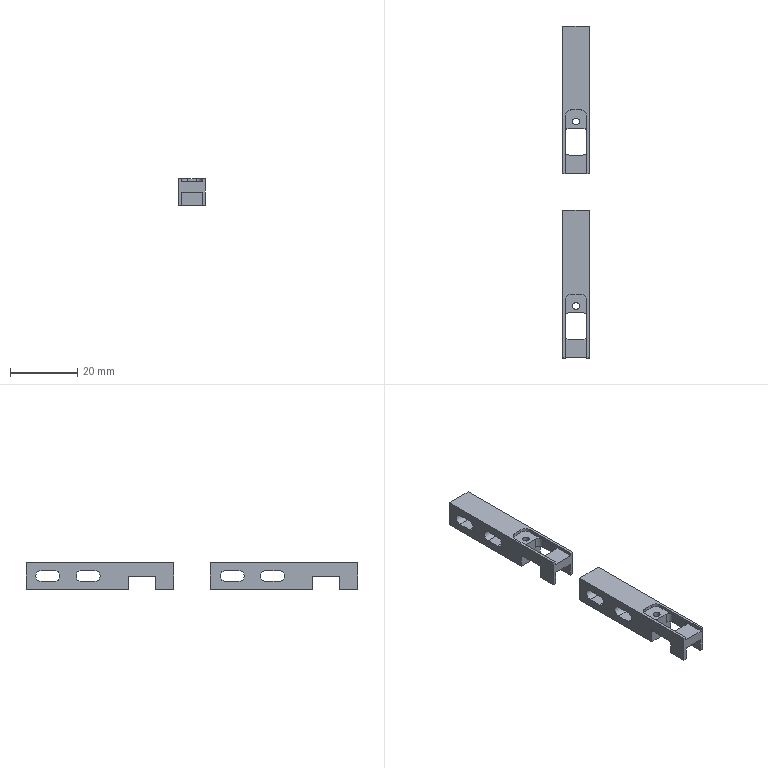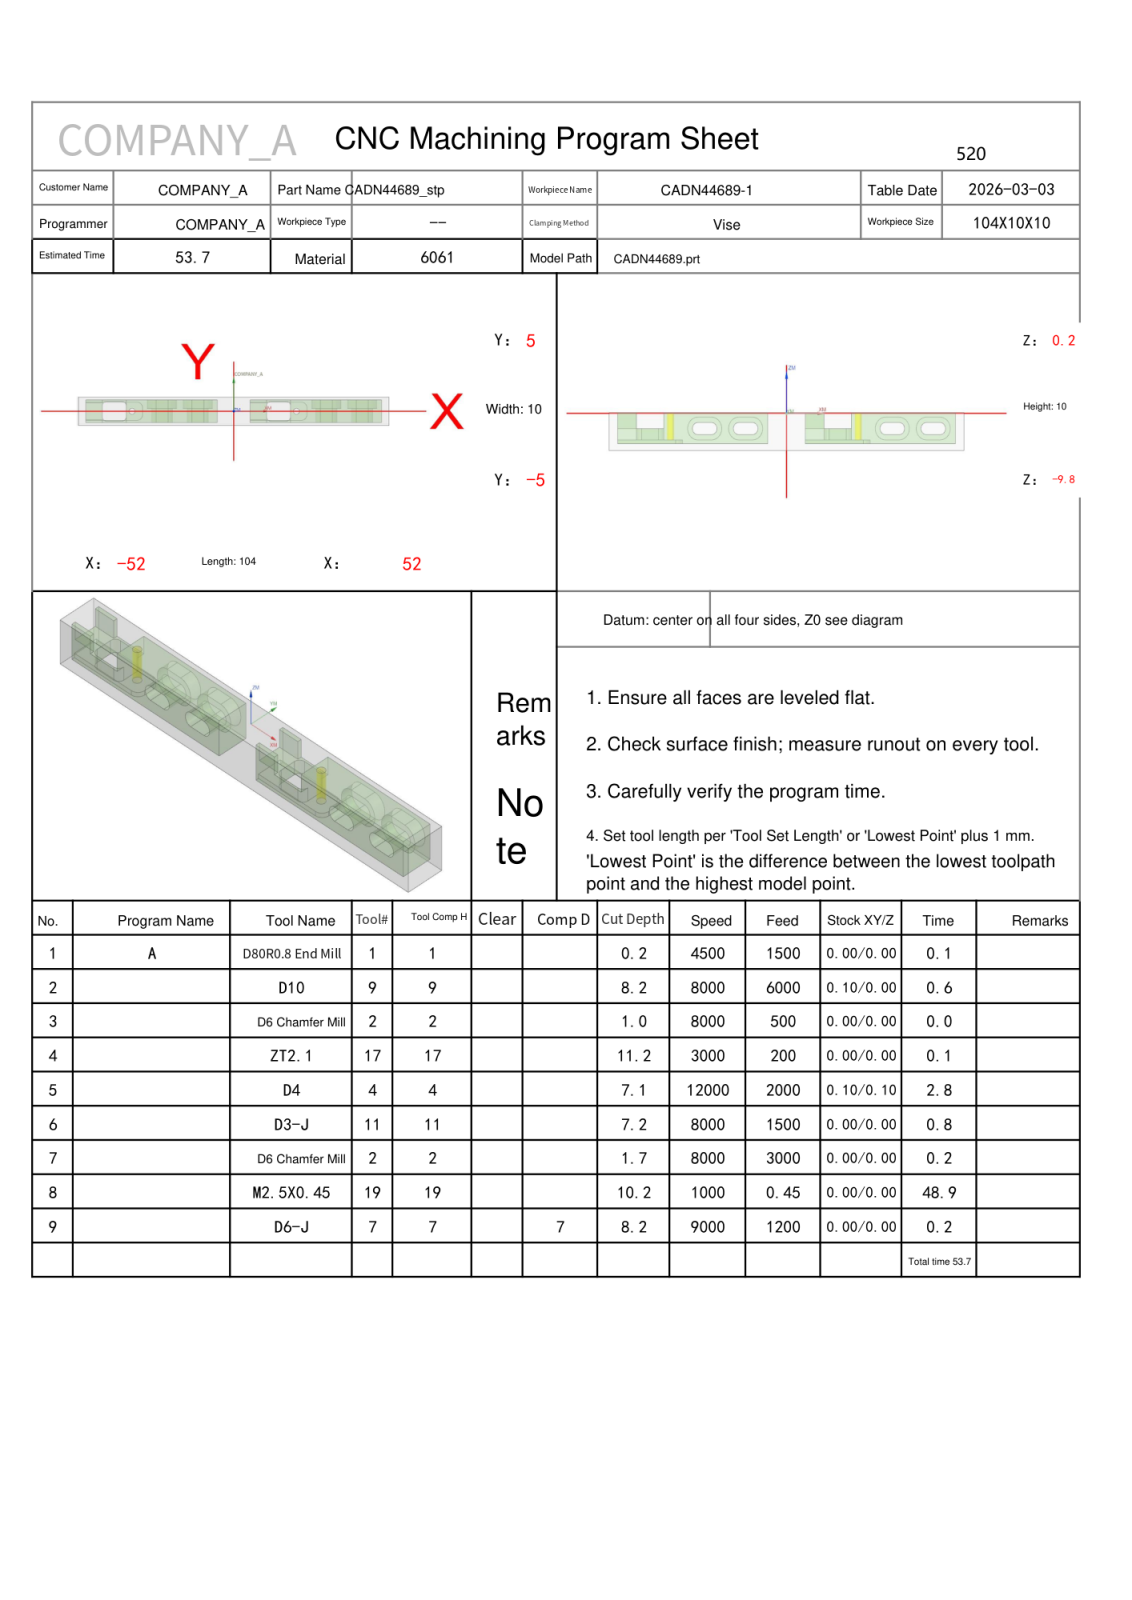NC program | NX | posted by the shop | part box 8 x 99 x 8 mm
Whole program:
%
O0001
(Machine time: 99.98 MIN)
(===Total Tool:8===)
(T1=D80R0.8 Indexable End Mill D=80.  R=0.8  D-  H01 Z=-0.   )
(T9=D10     D=10.  R=0.   D-  H09 Z=-8.   )
(T2=D6 Chamfer Mill   D=6.   R=0.   D-  H02 Z=-1.5  )
(T17=ZT2.1  D=2.1  DR_a=118 D-  H17 Z=-11.  )
(T4=D4      D=4.   R=0.   D-  H04 Z=-6.9  )
(T11=D3-J   D=3.   R=0.   D11 H11 Z=-7.   )
(T19=M2.5X0.45 D=2.05 DR_a=180 D-  H19 Z=-10.  )
(T7=D6-J    D=6.   R=0.   D7  H07 Z=-8.   )
G80 G90 G17 G49 G40
G91 G28 Z0
M01
N1 T01 M06
(D80R0.8 Indexable End Mill  D=80. R=0.8 H=01 ce=0.00 di=0.00)
G00 G90 G54 X-94.5 Y0.0 M03 S4500
G43 H01 Z50.
M08
Z2.
G01 Z0.0 F1500.
X-89.5
X89.5
X94.5
Z2.
G00 Z50.
G91 G28 Z0.0
M05
M09
G91 G28 Z0.0
M01
N2 T09 M06
(D10  D=10. R=0. H=09 ce=0.10 di=0.00)
G00 G90 G54 X27.5 Y-9.1 M03 S8000
G43 H09 Z50.
M08
Z.5
G01 X5.5 Z.375 F6000.
G02 X.4 Y-4. Z.33 I0.0 J5.1
G01 Y4. Z.284
G02 X5.5 Y9.1 Z.239 I5.1 J0.0
G01 X49.5 Z-.011
G02 X54.6 Y4. Z-.057 I0.0 J-5.1
G01 Y-4. Z-.102
G02 X49.5 Y-9.1 Z-.148 I-5.1 J0.0
G01 X5.5 Z-.398
G02 X.4 Y-4. Z-.443 I0.0 J5.1
G01 Y4. Z-.489
G02 X5.5 Y9.1 Z-.534 I5.1 J0.0
G01 X49.5 Z-.784
G02 X54.6 Y4. Z-.83 I0.0 J-5.1
G01 Y-4. Z-.875
G02 X49.5 Y-9.1 Z-.92 I-5.1 J0.0
G01 X5.5 Z-1.17
G02 X.4 Y-4. Z-1.216 I0.0 J5.1
G01 Y4. Z-1.261
G02 X5.5 Y9.1 Z-1.307 I5.1 J0.0
G01 X49.5 Z-1.557
G02 X54.6 Y4. Z-1.602 I0.0 J-5.1
G01 Y-4. Z-1.648
G02 X49.5 Y-9.1 Z-1.693 I-5.1 J0.0
G01 X5.5 Z-1.943
G02 X.4 Y-4. Z-1.989 I0.0 J5.1
G01 Y4. Z-2.034
G02 X5.5 Y9.1 Z-2.08 I5.1 J0.0
G01 X49.5 Z-2.33
G02 X54.6 Y4. Z-2.375 I0.0 J-5.1
G01 Y-4. Z-2.42
G02 X49.5 Y-9.1 Z-2.466 I-5.1 J0.0
G01 X5.5 Z-2.716
G02 X.4 Y-4. Z-2.761 I0.0 J5.1
G01 Y4. Z-2.807
G02 X5.5 Y9.1 Z-2.852 I5.1 J0.0
G01 X49.5 Z-3.102
G02 X54.6 Y4. Z-3.148 I0.0 J-5.1
G01 Y-4. Z-3.193
G02 X49.5 Y-9.1 Z-3.239 I-5.1 J0.0
G01 X5.5 Z-3.489
G02 X.4 Y-4. Z-3.534 I0.0 J5.1
G01 Y4. Z-3.58
G02 X5.5 Y9.1 Z-3.625 I5.1 J0.0
G01 X49.5 Z-3.875
G02 X54.6 Y4. Z-3.92 I0.0 J-5.1
G01 Y-4. Z-3.966
G02 X49.5 Y-9.1 Z-4.011 I-5.1 J0.0
G01 X5.5 Z-4.261
G02 X.4 Y-4. Z-4.307 I0.0 J5.1
G01 Y4. Z-4.352
G02 X5.5 Y9.1 Z-4.398 I5.1 J0.0
G01 X49.5 Z-4.648
G02 X54.6 Y4. Z-4.693 I0.0 J-5.1
G01 Y-4. Z-4.739
G02 X49.5 Y-9.1 Z-4.784 I-5.1 J0.0
G01 X5.5 Z-5.034
G02 X.4 Y-4. Z-5.08 I0.0 J5.1
G01 Y4. Z-5.125
G02 X5.5 Y9.1 Z-5.17 I5.1 J0.0
G01 X49.5 Z-5.42
G02 X54.6 Y4. Z-5.466 I0.0 J-5.1
G01 Y-4. Z-5.511
G02 X49.5 Y-9.1 Z-5.557 I-5.1 J0.0
G01 X5.5 Z-5.807
G02 X.4 Y-4. Z-5.852 I0.0 J5.1
G01 Y4. Z-5.898
G02 X5.5 Y9.1 Z-5.943 I5.1 J0.0
G01 X49.5 Z-6.193
G02 X54.6 Y4. Z-6.239 I0.0 J-5.1
G01 Y-4. Z-6.284
G02 X49.5 Y-9.1 Z-6.33 I-5.1 J0.0
G01 X5.5 Z-6.58
G02 X.4 Y-4. Z-6.625 I0.0 J5.1
G01 Y4. Z-6.67
G02 X5.5 Y9.1 Z-6.716 I5.1 J0.0
G01 X49.5 Z-6.966
G02 X54.6 Y4. Z-7.011 I0.0 J-5.1
G01 Y-4. Z-7.057
G02 X49.5 Y-9.1 Z-7.102 I-5.1 J0.0
G01 X5.5 Z-7.352
G02 X.4 Y-4. Z-7.398 I0.0 J5.1
G01 Y4. Z-7.443
G02 X5.5 Y9.1 Z-7.489 I5.1 J0.0
G01 X49.5 Z-7.739
G02 X54.6 Y4. Z-7.784 I0.0 J-5.1
G01 Y-4. Z-7.83
G02 X49.5 Y-9.1 Z-7.875 I-5.1 J0.0
G01 X27.5 Z-8.
X5.5
G02 X.4 Y-4. I0.0 J5.1
G01 Y4.
G02 X5.5 Y9.1 I5.1 J0.0
G01 X49.5
G02 X54.6 Y4. I0.0 J-5.1
G01 Y-4.
G02 X49.5 Y-9.1 I-5.1 J0.0
G01 X27.5
X27.
Z-7.
G00 Z50.
X-27.5
Z.5
G01 X-49.5 Z.375
G02 X-54.6 Y-4. Z.33 I0.0 J5.1
G01 Y4. Z.284
G02 X-49.5 Y9.1 Z.239 I5.1 J0.0
G01 X-5.5 Z-.011
G02 X-.4 Y4. Z-.057 I0.0 J-5.1
G01 Y-4. Z-.102
G02 X-5.5 Y-9.1 Z-.148 I-5.1 J0.0
G01 X-49.5 Z-.398
G02 X-54.6 Y-4. Z-.443 I0.0 J5.1
G01 Y4. Z-.489
G02 X-49.5 Y9.1 Z-.534 I5.1 J0.0
G01 X-5.5 Z-.784
G02 X-.4 Y4. Z-.83 I0.0 J-5.1
G01 Y-4. Z-.875
G02 X-5.5 Y-9.1 Z-.92 I-5.1 J0.0
G01 X-49.5 Z-1.17
G02 X-54.6 Y-4. Z-1.216 I0.0 J5.1
G01 Y4. Z-1.261
G02 X-49.5 Y9.1 Z-1.307 I5.1 J0.0
G01 X-5.5 Z-1.557
G02 X-.4 Y4. Z-1.602 I0.0 J-5.1
G01 Y-4. Z-1.648
G02 X-5.5 Y-9.1 Z-1.693 I-5.1 J0.0
G01 X-49.5 Z-1.943
G02 X-54.6 Y-4. Z-1.989 I0.0 J5.1
G01 Y4. Z-2.034
G02 X-49.5 Y9.1 Z-2.08 I5.1 J0.0
G01 X-5.5 Z-2.33
G02 X-.4 Y4. Z-2.375 I0.0 J-5.1
G01 Y-4. Z-2.42
G02 X-5.5 Y-9.1 Z-2.466 I-5.1 J0.0
G01 X-49.5 Z-2.716
G02 X-54.6 Y-4. Z-2.761 I0.0 J5.1
G01 Y4. Z-2.807
G02 X-49.5 Y9.1 Z-2.852 I5.1 J0.0
G01 X-5.5 Z-3.102
G02 X-.4 Y4. Z-3.148 I0.0 J-5.1
G01 Y-4. Z-3.193
G02 X-5.5 Y-9.1 Z-3.239 I-5.1 J0.0
G01 X-49.5 Z-3.489
G02 X-54.6 Y-4. Z-3.534 I0.0 J5.1
G01 Y4. Z-3.58
G02 X-49.5 Y9.1 Z-3.625 I5.1 J0.0
G01 X-5.5 Z-3.875
G02 X-.4 Y4. Z-3.92 I0.0 J-5.1
G01 Y-4. Z-3.966
G02 X-5.5 Y-9.1 Z-4.011 I-5.1 J0.0
G01 X-49.5 Z-4.261
G02 X-54.6 Y-4. Z-4.307 I0.0 J5.1
G01 Y4. Z-4.352
G02 X-49.5 Y9.1 Z-4.398 I5.1 J0.0
G01 X-5.5 Z-4.648
G02 X-.4 Y4. Z-4.693 I0.0 J-5.1
G01 Y-4. Z-4.739
G02 X-5.5 Y-9.1 Z-4.784 I-5.1 J0.0
G01 X-49.5 Z-5.034
G02 X-54.6 Y-4. Z-5.08 I0.0 J5.1
G01 Y4. Z-5.125
G02 X-49.5 Y9.1 Z-5.17 I5.1 J0.0
G01 X-5.5 Z-5.42
G02 X-.4 Y4. Z-5.466 I0.0 J-5.1
G01 Y-4. Z-5.511
G02 X-5.5 Y-9.1 Z-5.557 I-5.1 J0.0
G01 X-49.5 Z-5.807
G02 X-54.6 Y-4. Z-5.852 I0.0 J5.1
G01 Y4. Z-5.898
G02 X-49.5 Y9.1 Z-5.943 I5.1 J0.0
G01 X-5.5 Z-6.193
G02 X-.4 Y4. Z-6.239 I0.0 J-5.1
G01 Y-4. Z-6.284
G02 X-5.5 Y-9.1 Z-6.33 I-5.1 J0.0
G01 X-49.5 Z-6.58
G02 X-54.6 Y-4. Z-6.625 I0.0 J5.1
G01 Y4. Z-6.67
G02 X-49.5 Y9.1 Z-6.716 I5.1 J0.0
G01 X-5.5 Z-6.966
G02 X-.4 Y4. Z-7.011 I0.0 J-5.1
G01 Y-4. Z-7.057
G02 X-5.5 Y-9.1 Z-7.102 I-5.1 J0.0
G01 X-49.5 Z-7.352
G02 X-54.6 Y-4. Z-7.398 I0.0 J5.1
G01 Y4. Z-7.443
G02 X-49.5 Y9.1 Z-7.489 I5.1 J0.0
G01 X-5.5 Z-7.739
G02 X-.4 Y4. Z-7.784 I0.0 J-5.1
G01 Y-4. Z-7.83
G02 X-5.5 Y-9.1 Z-7.875 I-5.1 J0.0
G01 X-27.5 Z-8.
X-49.5
G02 X-54.6 Y-4. I0.0 J5.1
G01 Y4.
G02 X-49.5 Y9.1 I5.1 J0.0
G01 X-5.5
G02 X-.4 Y4. I0.0 J-5.1
G01 Y-4.
G02 X-5.5 Y-9.1 I-5.1 J0.0
G01 X-27.5
X-28.
Z-7.
G00 Z50.
G91 G28 Z0.0
M05
M09
G91 G28 Z0.0
M01
N3 T02 M06
(D6 Chamfer Mill  D=6. R=0. H=02 ce=0.00 di=0.00)
G00 G90 G54 X-34. Y0.0 M03 S8000
G43 H02 Z50.
M08
G98 G81 X-34. Y0.0 Z-.8 R1. F500.
X21.
G80
G00 Z50.
G91 G28 Z0.0
M05
M09
G91 G28 Z0.0
M01
N4 T17 M06
(ZT2.1 D=2.1 DR_a=118 H=17)
G00 G90 G54 X-34. Y0.0 M03 S3000
G43 H17 Z50.
M08
G98 G83 X-34. Y0.0 Z-11. R1. F200. Q2.
X21.
G80
G00 Z50.
G91 G28 Z0.0
M05
M09
G91 G28 Z0.0
M01
N5 T04 M06
(D4  D=4. R=0. H=04 ce=0.10 di=0.10)
G00 G90 G54 X-40. Y9.1 M03 S12000
G43 H04 Z50.
M08
Z.305
G01 Z-.195 F1000.
Y4.4
X-41.9
Y3.1
X-38.1
Y4.4
X-40.
X-40.5
Z.305
G00 Z.5
X-40. Y9.1
Z.11
G01 Z-.39
Y4.4
X-41.9
Y3.1
X-38.1
Y4.4
X-40.
X-40.5
Z.11
G00 Z.305
X-40. Y9.1
Z-.085
G01 Z-.585
Y4.4
X-41.9
Y3.1
X-38.1
Y4.4
X-40.
X-40.5
Z-.085
G00 Z.11
X-40. Y9.1
Z-.28
G01 Z-.78
Y4.4
X-41.9
Y3.1
X-38.1
Y4.4
X-40.
X-40.5
Z-.28
G00 Z-.085
X-40. Y9.1
Z-.475
G01 Z-.975
Y4.4
X-41.9
Y3.1
X-38.1
Y4.4
X-40.
X-40.5
Z-.475
G00 Z-.28
X-40. Y9.1
Z-.67
G01 Z-1.17
Y4.4
X-41.9
Y3.1
X-38.1
Y4.4
X-40.
X-40.5
Z-.67
G00 Z-.475
X-40. Y9.1
Z-.865
G01 Z-1.365
Y4.4
X-41.9
Y3.1
X-38.1
Y4.4
X-40.
X-40.5
Z-.865
G00 Z-.67
X-40. Y9.1
Z-1.06
G01 Z-1.56
Y4.4
X-41.9
Y3.1
X-38.1
Y4.4
X-40.
X-40.5
Z-1.06
G00 Z-.865
X-40. Y9.1
Z-1.255
G01 Z-1.755
Y4.4
X-41.9
Y3.1
X-38.1
Y4.4
X-40.
X-40.5
Z-1.255
G00 Z-1.06
X-40. Y9.1
Z-1.45
G01 Z-1.95
Y4.4
X-41.9
Y3.1
X-38.1
Y4.4
X-40.
X-40.5
Z-1.45
G00 Z-1.255
X-40. Y9.1
Z-1.645
G01 Z-2.145
Y4.4
X-41.9
Y3.1
X-38.1
Y4.4
X-40.
X-40.5
Z-1.645
G00 Z-1.45
X-40. Y9.1
Z-1.84
G01 Z-2.34
Y4.4
X-41.9
Y3.1
X-38.1
Y4.4
X-40.
X-40.5
Z-1.84
G00 Z-1.645
X-40. Y9.1
Z-2.035
G01 Z-2.535
Y4.4
X-41.9
Y3.1
X-38.1
Y4.4
X-40.
X-40.5
Z-2.035
G00 Z-1.84
X-40. Y9.1
Z-2.23
G01 Z-2.73
Y4.4
X-41.9
Y3.1
X-38.1
Y4.4
X-40.
X-40.5
Z-2.23
G00 Z-2.035
X-40. Y9.1
Z-2.425
G01 Z-2.925
Y4.4
X-41.9
Y3.1
X-38.1
Y4.4
X-40.
X-40.5
Z-2.425
G00 Z-2.23
X-40. Y9.1
Z-2.62
G01 Z-3.12
Y4.4
X-41.9
Y3.1
X-38.1
Y4.4
X-40.
X-40.5
Z-2.62
G00 Z-2.425
X-40. Y9.1
Z-2.815
G01 Z-3.315
Y4.4
X-41.9
Y3.1
X-38.1
Y4.4
X-40.
X-40.5
Z-2.815
G00 Z-2.62
X-40. Y9.1
Z-3.01
G01 Z-3.51
Y4.4
X-41.9
Y3.1
X-38.1
Y4.4
X-40.
X-40.5
Z-3.01
G00 Z-2.815
X-40. Y9.1
Z-3.205
G01 Z-3.705
Y4.4
X-41.9
Y3.1
X-38.1
Y4.4
X-40.
X-40.5
Z-3.205
G00 Z-3.01
X-40. Y9.1
Z-3.4
G01 Z-3.9
Y4.4
X-41.9
Y3.1
X-38.1
Y4.4
X-40.
X-40.5
Z-3.4
G00 Z50.
X-54.6 Y0.0
Z.305
G01 Z-.195
X-49.9
Y-.9
X-42.6
Y.9
X-49.9
Y0.0
Y-.5
Z.305
G00 Z50.
X-54.6 Y0.0
Z.11
G01 Z-.39
X-49.9
Y-.9
X-42.6
Y.9
X-49.9
Y0.0
Y-.5
Z.11
G00 Z.305
X-54.6 Y0.0
Z-.085
G01 Z-.585
X-49.9
Y-.9
X-42.6
Y.9
X-49.9
Y0.0
Y-.5
Z-.085
G00 Z.11
X-54.6 Y0.0
Z-.28
G01 Z-.78
X-49.9
Y-.9
X-42.6
Y.9
X-49.9
Y0.0
Y-.5
Z-.28
G00 Z-.085
X-54.6 Y0.0
Z-.475
G01 Z-.975
X-49.9
Y-.9
X-42.6
Y.9
X-49.9
Y0.0
Y-.5
Z-.475
G00 Z-.28
X-54.6 Y0.0
Z-.67
G01 Z-1.17
X-49.9
Y-.9
X-42.6
Y.9
X-49.9
Y0.0
Y-.5
Z-.67
G00 Z-.475
X-54.6 Y0.0
Z-.865
G01 Z-1.365
X-49.9
Y-.9
X-42.6
Y.9
X-49.9
Y0.0
Y-.5
Z-.865
G00 Z-.67
X-54.6 Y0.0
Z-1.06
G01 Z-1.56
X-49.9
Y-.9
X-42.6
Y.9
X-49.9
Y0.0
Y-.5
Z-1.06
G00 Z-.865
X-54.6 Y0.0
Z-1.255
G01 Z-1.755
X-49.9
Y-.9
X-42.6
Y.9
X-49.9
Y0.0
Y-.5
Z-1.255
G00 Z-1.06
X-54.6 Y0.0
Z-1.45
G01 Z-1.95
X-49.9
Y-.9
X-42.6
Y.9
X-49.9
Y0.0
Y-.5
Z-1.45
G00 Z-1.255
X-54.6 Y0.0
Z-1.645
G01 Z-2.145
X-49.9
Y-.9
X-42.6
Y.9
X-49.9
Y0.0
Y-.5
Z-1.645
G00 Z-1.45
X-54.6 Y0.0
Z-1.84
G01 Z-2.34
X-49.9
Y-.9
X-42.6
Y.9
X-49.9
Y0.0
Y-.5
Z-1.84
G00 Z-1.645
X-54.6 Y0.0
Z-2.035
G01 Z-2.535
X-49.9
Y-.9
X-42.6
Y.9
X-49.9
Y0.0
Y-.5
Z-2.035
G00 Z-1.84
X-54.6 Y0.0
Z-2.23
G01 Z-2.73
X-49.9
Y-.9
X-42.6
Y.9
X-49.9
Y0.0
Y-.5
Z-2.23
G00 Z-2.035
X-54.6 Y0.0
Z-2.425
G01 Z-2.925
X-49.9
Y-.9
X-42.6
Y.9
X-49.9
Y0.0
Y-.5
Z-2.425
G00 Z-2.23
X-54.6 Y0.0
Z-2.62
G01 Z-3.12
X-49.9
Y-.9
X-42.6
Y.9
X-49.9
Y0.0
Y-.5
Z-2.62
G00 Z-2.425
X-54.6 Y0.0
Z-2.815
G01 Z-3.315
X-49.9
Y-.9
X-42.6
Y.9
X-49.9
Y0.0
Y-.5
Z-2.815
G00 Z-2.62
X-54.6 Y0.0
Z-3.01
G01 Z-3.51
X-49.9
Y-.9
X-42.6
Y.9
X-49.9
Y0.0
Y-.5
Z-3.01
G00 Z-2.815
X-54.6 Y0.0
Z-3.205
G01 Z-3.705
X-49.9
Y-.9
X-42.6
Y.9
X-49.9
Y0.0
Y-.5
Z-3.205
G00 Z-3.01
X-54.6 Y0.0
Z-3.4
G01 Z-3.9
X-49.9
Y-.9
X-42.6
Y.9
X-49.9
Y0.0
Y-.5
Z-3.4
G00 Z50.
X-40. Y-9.1
Z.305
G01 Z-.195
Y-4.4
X-38.1
Y-3.1
X-41.9
Y-4.4
X-40.
X-39.5
Z.305
G00 Z.5
X-40. Y-9.1
Z.11
G01 Z-.39
Y-4.4
X-38.1
Y-3.1
X-41.9
Y-4.4
X-40.
X-39.5
Z.11
G00 Z.305
X-40. Y-9.1
Z-.085
G01 Z-.585
Y-4.4
X-38.1
Y-3.1
X-41.9
Y-4.4
X-40.
X-39.5
Z-.085
G00 Z.11
X-40. Y-9.1
Z-.28
G01 Z-.78
Y-4.4
X-38.1
Y-3.1
X-41.9
Y-4.4
X-40.
X-39.5
Z-.28
G00 Z-.085
X-40. Y-9.1
Z-.475
G01 Z-.975
Y-4.4
X-38.1
Y-3.1
X-41.9
Y-4.4
X-40.
X-39.5
Z-.475
G00 Z-.28
X-40. Y-9.1
Z-.67
G01 Z-1.17
Y-4.4
X-38.1
Y-3.1
X-41.9
Y-4.4
X-40.
X-39.5
Z-.67
G00 Z-.475
X-40. Y-9.1
Z-.865
G01 Z-1.365
Y-4.4
X-38.1
Y-3.1
X-41.9
Y-4.4
X-40.
X-39.5
Z-.865
G00 Z-.67
X-40. Y-9.1
Z-1.06
G01 Z-1.56
Y-4.4
X-38.1
Y-3.1
X-41.9
Y-4.4
X-40.
X-39.5
Z-1.06
G00 Z-.865
X-40. Y-9.1
Z-1.255
G01 Z-1.755
Y-4.4
X-38.1
Y-3.1
X-41.9
Y-4.4
X-40.
X-39.5
Z-1.255
G00 Z-1.06
X-40. Y-9.1
Z-1.45
G01 Z-1.95
Y-4.4
X-38.1
Y-3.1
X-41.9
Y-4.4
X-40.
X-39.5
Z-1.45
G00 Z-1.255
X-40. Y-9.1
Z-1.645
G01 Z-2.145
Y-4.4
X-38.1
Y-3.1
X-41.9
Y-4.4
X-40.
X-39.5
Z-1.645
G00 Z-1.45
X-40. Y-9.1
Z-1.84
G01 Z-2.34
Y-4.4
X-38.1
Y-3.1
X-41.9
Y-4.4
X-40.
X-39.5
Z-1.84
G00 Z-1.645
X-40. Y-9.1
Z-2.035
G01 Z-2.535
Y-4.4
X-38.1
Y-3.1
X-41.9
Y-4.4
X-40.
X-39.5
Z-2.035
G00 Z-1.84
X-40. Y-9.1
Z-2.23
G01 Z-2.73
Y-4.4
X-38.1
Y-3.1
X-41.9
Y-4.4
X-40.
X-39.5
Z-2.23
G00 Z-2.035
X-40. Y-9.1
Z-2.425
G01 Z-2.925
Y-4.4
X-38.1
Y-3.1
X-41.9
Y-4.4
X-40.
X-39.5
Z-2.425
G00 Z-2.23
X-40. Y-9.1
Z-2.62
G01 Z-3.12
Y-4.4
X-38.1
Y-3.1
X-41.9
Y-4.4
X-40.
X-39.5
Z-2.62
G00 Z-2.425
X-40. Y-9.1
Z-2.815
G01 Z-3.315
Y-4.4
X-38.1
Y-3.1
X-41.9
Y-4.4
X-40.
X-39.5
Z-2.815
G00 Z-2.62
X-40. Y-9.1
Z-3.01
G01 Z-3.51
Y-4.4
X-38.1
Y-3.1
X-41.9
Y-4.4
X-40.
X-39.5
Z-3.01
G00 Z-2.815
X-40. Y-9.1
Z-3.205
G01 Z-3.705
Y-4.4
X-38.1
Y-3.1
X-41.9
Y-4.4
X-40.
X-39.5
Z-3.205
G00 Z-3.01
X-40. Y-9.1
Z-3.4
G01 Z-3.9
Y-4.4
X-38.1
Y-3.1
X-41.9
Y-4.4
X-40.
X-39.5
Z-3.4
G00 Z50.
X15. Y9.1
Z.305
G01 Z-.195
Y4.4
X13.1
Y3.1
X16.9
Y4.4
X15.
X14.5
Z.305
G00 Z.5
X15. Y9.1
Z.11
G01 Z-.39
Y4.4
X13.1
Y3.1
X16.9
Y4.4
X15.
X14.5
Z.11
G00 Z.305
X15. Y9.1
Z-.085
G01 Z-.585
Y4.4
X13.1
Y3.1
X16.9
Y4.4
X15.
X14.5
Z-.085
G00 Z.11
X15. Y9.1
Z-.28
G01 Z-.78
Y4.4
X13.1
Y3.1
X16.9
Y4.4
X15.
X14.5
Z-.28
G00 Z-.085
X15. Y9.1
Z-.475
G01 Z-.975
Y4.4
X13.1
Y3.1
X16.9
Y4.4
X15.
X14.5
Z-.475
G00 Z-.28
X15. Y9.1
Z-.67
G01 Z-1.17
Y4.4
X13.1
Y3.1
X16.9
Y4.4
X15.
X14.5
Z-.67
G00 Z-.475
X15. Y9.1
Z-.865
G01 Z-1.365
Y4.4
X13.1
Y3.1
X16.9
Y4.4
X15.
X14.5
Z-.865
G00 Z-.67
X15. Y9.1
Z-1.06
G01 Z-1.56
Y4.4
X13.1
Y3.1
X16.9
Y4.4
X15.
X14.5
Z-1.06
G00 Z-.865
X15. Y9.1
Z-1.255
G01 Z-1.755
Y4.4
X13.1
Y3.1
X16.9
Y4.4
X15.
X14.5
Z-1.255
G00 Z-1.06
X15. Y9.1
Z-1.45
G01 Z-1.95
Y4.4
X13.1
Y3.1
X16.9
Y4.4
X15.
X14.5
Z-1.45
G00 Z-1.255
X15. Y9.1
Z-1.645
G01 Z-2.145
Y4.4
X13.1
Y3.1
X16.9
Y4.4
X15.
X14.5
Z-1.645
G00 Z-1.45
X15. Y9.1
Z-1.84
G01 Z-2.34
Y4.4
X13.1
Y3.1
X16.9
Y4.4
X15.
X14.5
Z-1.84
G00 Z-1.645
X15. Y9.1
Z-2.035
G01 Z-2.535
Y4.4
X13.1
Y3.1
X16.9
Y4.4
X15.
X14.5
Z-2.035
G00 Z-1.84
X15. Y9.1
Z-2.23
G01 Z-2.73
Y4.4
X13.1
Y3.1
X16.9
Y4.4
X15.
X14.5
Z-2.23
G00 Z-2.035
X15. Y9.1
Z-2.425
G01 Z-2.925
Y4.4
X13.1
Y3.1
X16.9
Y4.4
X15.
X14.5
Z-2.425
G00 Z-2.23
X15. Y9.1
Z-2.62
G01 Z-3.12
Y4.4
X13.1
Y3.1
X16.9
Y4.4
X15.
X14.5
Z-2.62
G00 Z-2.425
X15. Y9.1
Z-2.815
G01 Z-3.315
Y4.4
X13.1
Y3.1
X16.9
Y4.4
X15.
X14.5
Z-2.815
G00 Z-2.62
X15. Y9.1
Z-3.01
G01 Z-3.51
Y4.4
X13.1
Y3.1
X16.9
Y4.4
X15.
X14.5
Z-3.01
G00 Z-2.815
X15. Y9.1
Z-3.205
G01 Z-3.705
Y4.4
X13.1
Y3.1
X16.9
Y4.4
X15.
X14.5
Z-3.205
G00 Z-3.01
X15. Y9.1
Z-3.4
G01 Z-3.9
Y4.4
X13.1
Y3.1
X16.9
Y4.4
X15.
X14.5
Z-3.4
G00 Z50.
X.4 Y0.0
Z.305
G01 Z-.195
X5.1
Y-.9
X12.4
Y.9
X5.1
Y0.0
Y-.5
Z.305
G00 Z50.
X.4 Y0.0
Z.11
G01 Z-.39
X5.1
Y-.9
X12.4
Y.9
X5.1
Y0.0
Y-.5
Z.11
G00 Z.305
X.4 Y0.0
Z-.085
G01 Z-.585
X5.1
Y-.9
X12.4
Y.9
X5.1
Y0.0
Y-.5
Z-.085
G00 Z.11
X.4 Y0.0
Z-.28
G01 Z-.78
X5.1
Y-.9
X12.4
Y.9
X5.1
Y0.0
Y-.5
Z-.28
G00 Z-.085
X.4 Y0.0
Z-.475
G01 Z-.975
X5.1
Y-.9
X12.4
Y.9
X5.1
Y0.0
Y-.5
Z-.475
G00 Z-.28
X.4 Y0.0
Z-.67
G01 Z-1.17
X5.1
Y-.9
X12.4
Y.9
X5.1
Y0.0
Y-.5
Z-.67
G00 Z-.475
X.4 Y0.0
Z-.865
G01 Z-1.365
X5.1
Y-.9
X12.4
Y.9
X5.1
Y0.0
Y-.5
Z-.865
G00 Z-.67
X.4 Y0.0
Z-1.06
G01 Z-1.56
X5.1
Y-.9
X12.4
Y.9
X5.1
Y0.0
Y-.5
Z-1.06
G00 Z-.865
X.4 Y0.0
Z-1.255
G01 Z-1.755
X5.1
Y-.9
X12.4
Y.9
X5.1
Y0.0
Y-.5
Z-1.255
G00 Z-1.06
X.4 Y0.0
Z-1.45
G01 Z-1.95
X5.1
Y-.9
X12.4
Y.9
X5.1
Y0.0
Y-.5
Z-1.45
G00 Z-1.255
X.4 Y0.0
Z-1.645
G01 Z-2.145
X5.1
Y-.9
X12.4
Y.9
X5.1
Y0.0
Y-.5
Z-1.645
G00 Z-1.45
X.4 Y0.0
Z-1.84
G01 Z-2.34
X5.1
Y-.9
X12.4
Y.9
X5.1
Y0.0
Y-.5
Z-1.84
G00 Z-1.645
X.4 Y0.0
Z-2.035
G01 Z-2.535
X5.1
Y-.9
X12.4
Y.9
X5.1
Y0.0
Y-.5
Z-2.035
G00 Z-1.84
X.4 Y0.0
Z-2.23
G01 Z-2.73
X5.1
Y-.9
X12.4
Y.9
X5.1
Y0.0
Y-.5
Z-2.23
G00 Z-2.035
X.4 Y0.0
Z-2.425
G01 Z-2.925
X5.1
Y-.9
X12.4
Y.9
X5.1
Y0.0
Y-.5
Z-2.425
G00 Z-2.23
X.4 Y0.0
Z-2.62
G01 Z-3.12
X5.1
Y-.9
X12.4
Y.9
X5.1
Y0.0
Y-.5
Z-2.62
G00 Z-2.425
X.4 Y0.0
Z-2.815
G01 Z-3.315
X5.1
Y-.9
X12.4
Y.9
X5.1
Y0.0
Y-.5
Z-2.815
G00 Z-2.62
X.4 Y0.0
Z-3.01
G01 Z-3.51
X5.1
Y-.9
X12.4
Y.9
X5.1
Y0.0
Y-.5
Z-3.01
G00 Z-2.815
X.4 Y0.0
Z-3.205
G01 Z-3.705
X5.1
Y-.9
X12.4
Y.9
X5.1
Y0.0
Y-.5
Z-3.205
G00 Z-3.01
X.4 Y0.0
Z-3.4
G01 Z-3.9
X5.1
Y-.9
X12.4
Y.9
X5.1
Y0.0
Y-.5
Z-3.4
G00 Z50.
X15. Y-9.1
Z.305
G01 Z-.195
Y-4.4
X16.9
Y-3.1
X13.1
Y-4.4
X15.
X15.5
Z.305
G00 Z.5
X15. Y-9.1
Z.11
G01 Z-.39
Y-4.4
X16.9
Y-3.1
X13.1
Y-4.4
X15.
X15.5
Z.11
G00 Z.305
X15. Y-9.1
Z-.085
G01 Z-.585
Y-4.4
X16.9
Y-3.1
X13.1
Y-4.4
X15.
X15.5
Z-.085
G00 Z.11
X15. Y-9.1
Z-.28
G01 Z-.78
Y-4.4
X16.9
Y-3.1
X13.1
Y-4.4
X15.
X15.5
Z-.28
G00 Z-.085
X15. Y-9.1
Z-.475
G01 Z-.975
Y-4.4
X16.9
Y-3.1
X13.1
Y-4.4
X15.
X15.5
Z-.475
G00 Z-.28
X15. Y-9.1
Z-.67
G01 Z-1.17
Y-4.4
X16.9
Y-3.1
X13.1
Y-4.4
X15.
X15.5
Z-.67
G00 Z-.475
X15. Y-9.1
Z-.865
G01 Z-1.365
Y-4.4
X16.9
Y-3.1
X13.1
Y-4.4
X15.
X15.5
Z-.865
G00 Z-.67
X15. Y-9.1
Z-1.06
G01 Z-1.56
Y-4.4
X16.9
Y-3.1
X13.1
Y-4.4
X15.
X15.5
Z-1.06
G00 Z-.865
X15. Y-9.1
Z-1.255
G01 Z-1.755
Y-4.4
X16.9
Y-3.1
X13.1
Y-4.4
X15.
X15.5
Z-1.255
G00 Z-1.06
X15. Y-9.1
Z-1.45
G01 Z-1.95
Y-4.4
X16.9
Y-3.1
X13.1
Y-4.4
X15.
X15.5
Z-1.45
G00 Z-1.255
X15. Y-9.1
Z-1.645
G01 Z-2.145
Y-4.4
X16.9
Y-3.1
X13.1
Y-4.4
X15.
X15.5
Z-1.645
G00 Z-1.45
X15. Y-9.1
Z-1.84
G01 Z-2.34
Y-4.4
X16.9
Y-3.1
X13.1
Y-4.4
X15.
X15.5
Z-1.84
G00 Z-1.645
X15. Y-9.1
Z-2.035
G01 Z-2.535
Y-4.4
X16.9
Y-3.1
X13.1
Y-4.4
X15.
X15.5
Z-2.035
G00 Z-1.84
X15. Y-9.1
Z-2.23
G01 Z-2.73
Y-4.4
X16.9
Y-3.1
X13.1
Y-4.4
X15.
X15.5
Z-2.23
G00 Z-2.035
X15. Y-9.1
Z-2.425
G01 Z-2.925
Y-4.4
X16.9
Y-3.1
X13.1
Y-4.4
X15.
X15.5
Z-2.425
G00 Z-2.23
X15. Y-9.1
Z-2.62
G01 Z-3.12
Y-4.4
X16.9
Y-3.1
X13.1
Y-4.4
X15.
X15.5
Z-2.62
G00 Z-2.425
X15. Y-9.1
Z-2.815
G01 Z-3.315
Y-4.4
X16.9
Y-3.1
X13.1
Y-4.4
X15.
X15.5
Z-2.815
G00 Z-2.62
X15. Y-9.1
Z-3.01
G01 Z-3.51
Y-4.4
X16.9
Y-3.1
X13.1
Y-4.4
X15.
X15.5
Z-3.01
G00 Z-2.815
X15. Y-9.1
Z-3.205
G01 Z-3.705
Y-4.4
X16.9
Y-3.1
X13.1
Y-4.4
X15.
X15.5
Z-3.205
G00 Z-3.01
X15. Y-9.1
Z-3.4
G01 Z-3.9
Y-4.4
X16.9
Y-3.1
X13.1
Y-4.4
X15.
X15.5
Z-3.4
G00 Z50.
G00 G90 X13.819 Y-1.4 M03 S8000
Z50.
Z1.
G01 X16.9 Z.839 F2000.
Y1.4 Z.692
X13.1 Z.493
Y-1.4 Z.346
X16.9 Z.147
Y1.4 Z0.0
X13.1 Z-.083
Y-1.4 Z-.144
X16.9 Z-.227
Y1.4 Z-.288
X13.1 Z-.37
Y-1.4 Z-.431
X16.9 Z-.514
Y1.4 Z-.575
X13.1 Z-.658
Y-1.4 Z-.719
X16.9 Z-.802
Y1.4 Z-.863
X13.1 Z-.945
Y-1.4 Z-1.006
X16.9 Z-1.089
Y1.4 Z-1.15
X13.1 Z-1.233
Y-1.4 Z-1.294
X16.9 Z-1.377
Y1.4 Z-1.438
X13.1 Z-1.52
Y-1.4 Z-1.581
X16.9 Z-1.664
Y1.4 Z-1.725
X13.1 Z-1.808
Y-1.4 Z-1.869
X16.9 Z-1.952
Y1.4 Z-2.013
X13.1 Z-2.095
Y-1.4 Z-2.156
X16.9 Z-2.239
Y1.4 Z-2.3
X13.1 Z-2.383
Y-1.4 Z-2.444
X16.9 Z-2.527
Y1.4 Z-2.588
X13.1 Z-2.67
Y-1.4 Z-2.731
X16.9 Z-2.814
Y1.4 Z-2.875
X13.1 Z-2.958
Y-1.4 Z-3.019
X16.9 Z-3.102
Y1.4 Z-3.163
X13.1 Z-3.245
Y-1.4 Z-3.306
X16.9 Z-3.389
Y1.4 Z-3.45
X13.1 Z-3.533
Y-1.4 Z-3.594
X16.9 Z-3.677
Y1.4 Z-3.738
X13.1 Z-3.82
Y-1.4 Z-3.881
X16.9 Z-3.964
Y1.4 Z-4.025
X13.1 Z-4.108
Y-1.4 Z-4.169
X16.9 Z-4.252
Y1.4 Z-4.313
X13.1 Z-4.395
Y-1.4 Z-4.456
X16.9 Z-4.539
Y1.4 Z-4.6
X13.1 Z-4.683
Y-1.4 Z-4.744
X16.9 Z-4.827
Y1.4 Z-4.888
X13.1 Z-4.97
Y-1.4 Z-5.031
X16.9 Z-5.114
Y1.4 Z-5.175
X13.1 Z-5.258
Y-1.4 Z-5.319
X16.9 Z-5.402
Y1.4 Z-5.463
X13.1 Z-5.545
Y-1.4 Z-5.606
X16.9 Z-5.689
Y1.4 Z-5.75
X13.1 Z-5.833
Y-1.4 Z-5.894
X16.9 Z-5.977
Y1.4 Z-6.038
X13.1 Z-6.12
Y-1.4 Z-6.181
X16.9 Z-6.264
Y1.4 Z-6.325
X13.1 Z-6.408
Y-1.4 Z-6.469
X16.9 Z-6.552
Y1.4 Z-6.613
X13.1 Z-6.695
Y-1.4 Z-6.756
X16.9 Z-6.839
Y1.4 Z-6.9
X13.1
Y-1.4
X16.9
Y1.4
X16.5
Z-5.9
G00 Z50.
X-38.819
Z1.
G01 X-41.9 Z.839
Y-1.4 Z.692
X-38.1 Z.493
Y1.4 Z.346
X-41.9 Z.147
Y-1.4 Z0.0
X-38.1 Z-.083
Y1.4 Z-.144
X-41.9 Z-.227
Y-1.4 Z-.288
X-38.1 Z-.37
Y1.4 Z-.431
X-41.9 Z-.514
Y-1.4 Z-.575
X-38.1 Z-.658
Y1.4 Z-.719
X-41.9 Z-.802
Y-1.4 Z-.863
X-38.1 Z-.945
Y1.4 Z-1.006
X-41.9 Z-1.089
Y-1.4 Z-1.15
X-38.1 Z-1.233
Y1.4 Z-1.294
X-41.9 Z-1.377
Y-1.4 Z-1.438
X-38.1 Z-1.52
Y1.4 Z-1.581
X-41.9 Z-1.664
Y-1.4 Z-1.725
X-38.1 Z-1.808
Y1.4 Z-1.869
X-41.9 Z-1.952
Y-1.4 Z-2.013
X-38.1 Z-2.095
Y1.4 Z-2.156
X-41.9 Z-2.239
Y-1.4 Z-2.3
X-38.1 Z-2.383
Y1.4 Z-2.444
X-41.9 Z-2.527
Y-1.4 Z-2.588
X-38.1 Z-2.67
Y1.4 Z-2.731
X-41.9 Z-2.814
Y-1.4 Z-2.875
X-38.1 Z-2.958
Y1.4 Z-3.019
X-41.9 Z-3.102
Y-1.4 Z-3.163
X-38.1 Z-3.245
Y1.4 Z-3.306
X-41.9 Z-3.389
Y-1.4 Z-3.45
X-38.1 Z-3.533
Y1.4 Z-3.594
X-41.9 Z-3.677
Y-1.4 Z-3.738
X-38.1 Z-3.82
Y1.4 Z-3.881
X-41.9 Z-3.964
Y-1.4 Z-4.025
X-38.1 Z-4.108
Y1.4 Z-4.169
X-41.9 Z-4.252
Y-1.4 Z-4.313
X-38.1 Z-4.395
Y1.4 Z-4.456
X-41.9 Z-4.539
Y-1.4 Z-4.6
X-38.1 Z-4.683
Y1.4 Z-4.744
X-41.9 Z-4.827
Y-1.4 Z-4.888
X-38.1 Z-4.97
Y1.4 Z-5.031
X-41.9 Z-5.114
Y-1.4 Z-5.175
X-38.1 Z-5.258
Y1.4 Z-5.319
X-41.9 Z-5.402
Y-1.4 Z-5.463
X-38.1 Z-5.545
Y1.4 Z-5.606
X-41.9 Z-5.689
Y-1.4 Z-5.75
X-38.1 Z-5.833
Y1.4 Z-5.894
X-41.9 Z-5.977
Y-1.4 Z-6.038
X-38.1 Z-6.12
Y1.4 Z-6.181
X-41.9 Z-6.264
Y-1.4 Z-6.325
X-38.1 Z-6.408
Y1.4 Z-6.469
X-41.9 Z-6.552
Y-1.4 Z-6.613
X-38.1 Z-6.695
Y1.4 Z-6.756
X-41.9 Z-6.839
Y-1.4 Z-6.9
X-38.1
Y1.4
X-41.9
Y-1.4
X-41.5
Z-5.9
G00 Z50.
G91 G28 Z0.0
M05
M09
G91 G28 Z0.0
M01
N6 T11 M06
(D3-J  D=3. R=0. H=11 ce=0.40 di=0.00)
G00 G90 G54 X-52. Y-.6 M03 S7000
G43 H11 Z10.4
M08
Z-2.5
G01 Z-4. F1500.
X-50.4
G03 X-49.8 Y0.0 I0.0 J.6
G01 Y.801
G02 X-49.501 Y1.1 I.3 J-.001
G01 X-43.999
G02 X-43.7 Y.801 I-.001 J-.3
G01 Y-.801
G02 X-43.999 Y-1.1 I-.3 J.001
G01 X-49.501
G02 X-49.8 Y-.801 I.001 J.3
G01 Y0.0
Y.801
X-49.802 Y.869
X-49.78 Y.933
X-49.736 Y.986
G03 X-49.537 Y1.1 I-.039 J.297
G01 X-51.6 Y.5
Z-2.5
G00 Z10.4
X-39.4 Y-6.1
Z-2.5
G01 Z-4.
Y-4.9
G03 X-40. Y-4.3 I-.6 J0.0
G01 X-41.801
G02 X-42.1 Y-4.001 I.001 J.3
G01 Y-3.499
G02 X-41.801 Y-3.2 I.3 J-.001
G01 X-38.199
G02 X-37.9 Y-3.499 I-.001 J-.3
G01 Y-4.001
G02 X-38.199 Y-4.3 I-.3 J.001
G01 X-40.
X-41.
G03 X-41.6 Y-4.9 I0.0 J-.6
G01 Y-6.5
Z-2.5
G00 Z0.0
X-40.6 Y6.1
Z-2.5
G01 Z-4.
Y4.9
G03 X-40. Y4.3 I.6 J0.0
G01 X-38.199
G02 X-37.9 Y4.001 I-.001 J-.3
G01 Y3.499
G02 X-38.199 Y3.2 I-.3 J.001
G01 X-41.801
G02 X-42.1 Y3.499 I.001 J.3
G01 Y4.001
G02 X-41.801 Y4.3 I.3 J-.001
G01 X-40.
X-39.
G03 X-38.4 Y4.9 I0.0 J.6
G01 Y6.5
Z-2.5
G00 Z10.4
X3. Y-.6
Z-2.5
G01 Z-4.
X4.6
G03 X5.2 Y0.0 I0.0 J.6
G01 Y.801
G02 X5.499 Y1.1 I.3 J-.001
G01 X11.001
G02 X11.3 Y.801 I-.001 J-.3
G01 Y-.801
G02 X11.001 Y-1.1 I-.3 J.001
G01 X5.499
G02 X5.2 Y-.801 I.001 J.3
G01 Y0.0
Y.801
X5.198 Y.869
X5.22 Y.933
X5.264 Y.986
G03 X5.463 Y1.1 I-.039 J.297
G01 X3.4 Y.5
Z-2.5
G00 Z10.4
X15.6 Y-6.1
Z-2.5
G01 Z-4.
Y-4.9
G03 X15. Y-4.3 I-.6 J0.0
G01 X13.199
G02 X12.9 Y-4.001 I.001 J.3
G01 Y-3.499
G02 X13.199 Y-3.2 I.3 J-.001
G01 X16.801
G02 X17.1 Y-3.499 I-.001 J-.3
G01 Y-4.001
G02 X16.801 Y-4.3 I-.3 J.001
G01 X15.
X14.
G03 X13.4 Y-4.9 I0.0 J-.6
G01 Y-6.5
Z-2.5
G00 Z0.0
X14.4 Y6.1
Z-2.5
G01 Z-4.
Y4.9
G03 X15. Y4.3 I.6 J0.0
G01 X16.801
G02 X17.1 Y4.001 I-.001 J-.3
G01 Y3.499
G02 X16.801 Y3.2 I-.3 J.001
G01 X13.199
G02 X12.9 Y3.499 I.001 J.3
G01 Y4.001
G02 X13.199 Y4.3 I.3 J-.001
G01 X15.
X16.
G03 X16.6 Y4.9 I0.0 J.6
G01 Y6.5
Z-2.5
G00 Z10.4
G00 G90 X16.4 Y-6.35 M03 S8000
Z50.
Z-3.495
G01 Z-3.995 F800.
G41 D11
X16.5
G03 X17.5 Y-5.35 I0.0 J1.
G01 Y5.35
G03 X16.5 Y6.35 I-1. J0.0
G01 G40 X16.4
Z-3.495
G00 Z50.
X13.6
Z-3.495
G01 Z-3.995
G41 D11
X13.5
G03 X12.5 Y5.35 I0.0 J-1.
G01 Y1.5
X4.15
G03 X3.15 Y.5 I0.0 J-1.
G01 G40 Y.4
Y-.4
G41 D11
Y-.5
G03 X4.15 Y-1.5 I1. J0.0
G01 X12.5
Y-5.35
G03 X13.5 Y-6.35 I1. J0.0
G01 G40 X13.6
Z-3.495
G00 Z50.
X-38.6
Z-3.495
G01 Z-3.995
G41 D11
X-38.5
G03 X-37.5 Y-5.35 I0.0 J1.
G01 Y5.35
G03 X-38.5 Y6.35 I-1. J0.0
G01 G40 X-38.6
Z-3.495
G00 Z50.
X-41.4
Z-3.495
G01 Z-3.995
G41 D11
X-41.5
G03 X-42.5 Y5.35 I0.0 J-1.
G01 Y1.5
X-50.85
G03 X-51.85 Y.5 I0.0 J-1.
G01 G40 Y.4
Y-.4
G41 D11
Y-.5
G03 X-50.85 Y-1.5 I1. J0.0
G01 X-42.5
Y-5.35
G03 X-41.5 Y-6.35 I1. J0.0
G01 G40 X-41.4
Z-3.495
G00 Z50.
G00 G90 X17.5 Y1.409 M03 S8000
Z50.
Z.5
G01 Y2. Z.469 F600.
X12.5 Z.207
Y-1.95 Z0.0
G41 D11
Y-2.
X17.5 Z-.278
Y2. Z-.5
X12.5 Z-.778
Y-2. Z-1.
X17.5 Z-1.278
Y2. Z-1.5
X12.5 Z-1.778
Y-2. Z-2.
X17.5 Z-2.278
Y2. Z-2.5
X12.5 Z-2.778
Y-2. Z-3.
X17.5 Z-3.278
Y2. Z-3.5
X12.5 Z-3.778
Y-2. Z-4.
X17.5 Z-4.278
Y2. Z-4.5
X12.5 Z-4.778
Y-2. Z-5.
X17.5 Z-5.278
Y2. Z-5.5
X12.5 Z-5.778
Y-2. Z-6.
X17.5 Z-6.278
Y2. Z-6.5
X12.5 Z-6.778
Y-2. Z-7.
X17.5
Y2.
X12.5
Y-2.
X12.9
X12.928 Y-1.998
X12.948 Y-1.978
X12.95 Y-1.95
G40 Y-1.9
Z-6.
G00 Z50.
X-37.5 Y1.409
Z.5
G01 Y2. Z.469
X-42.5 Z.207
Y-1.95 Z0.0
G41 D11
Y-2.
X-37.5 Z-.278
Y2. Z-.5
X-42.5 Z-.778
Y-2. Z-1.
X-37.5 Z-1.278
Y2. Z-1.5
X-42.5 Z-1.778
Y-2. Z-2.
X-37.5 Z-2.278
Y2. Z-2.5
X-42.5 Z-2.778
Y-2. Z-3.
X-37.5 Z-3.278
Y2. Z-3.5
X-42.5 Z-3.778
Y-2. Z-4.
X-37.5 Z-4.278
Y2. Z-4.5
X-42.5 Z-4.778
Y-2. Z-5.
X-37.5 Z-5.278
Y2. Z-5.5
X-42.5 Z-5.778
Y-2. Z-6.
X-37.5 Z-6.278
Y2. Z-6.5
X-42.5 Z-6.778
Y-2. Z-7.
X-37.5
Y2.
X-42.5
Y-2.
X-42.1
X-42.073 Y-1.998
X-42.052 Y-1.978
X-42.05 Y-1.95
G40 Y-1.9
Z-6.
G00 Z50.
G91 G28 Z0.0
M05
M09
G91 G28 Z0.0
M01
N7 T02 M06
(D6 Chamfer Mill  D=6. R=0. H=02 ce=0.00 di=0.00)
G00 G90 G54 X34.5 Y-6.128 M03 S8000
G43 H02 Z50.
M08
Z2.099
G01 Z-1.5 F3000.
G03 X34.58 Y-5.828 I-.52 J.3
X34.28 Y-5.308 I-.6 J0.0
G01 X34.25 Y-5.3
X19.
G02 X17.7 Y-4. I0.0 J1.3
G01 Y4.
G02 X19. Y5.3 I1.3 J0.0
G01 X49.5
G02 X50.8 Y4. I0.0 J-1.3
G01 Y-4.
G02 X49.5 Y-5.3 I-1.3 J0.0
G01 X34.25
X34.22 Y-5.308
G03 X33.92 Y-5.828 I.3 J-.52
X34. Y-6.128 I.6 J0.0
G01 Z2.099
G00 Z50.
X8. Y6.128
Z2.099
G01 Z-1.5
G03 X7.92 Y5.828 I.52 J-.3
X8.22 Y5.308 I.6 J0.0
G01 X8.25 Y5.3
X11.
G02 X12.3 Y4. I0.0 J-1.3
G01 Y3.
G02 X11. Y1.7 I-1.3 J0.0
G01 X5.5
G02 X4.2 Y3. I0.0 J1.3
G01 Y4.
G02 X5.5 Y5.3 I1.3 J0.0
G01 X8.25
X8.28 Y5.308
G03 X8.58 Y5.828 I-.3 J.52
X8.5 Y6.128 I-.6 J0.0
G01 Z2.099
G00 Z50.
Y-6.128
Z2.099
G01 Z-1.5
G03 X8.58 Y-5.828 I-.52 J.3
X8.28 Y-5.308 I-.6 J0.0
G01 X8.25 Y-5.3
X5.5
G02 X4.2 Y-4. I0.0 J1.3
G01 Y-3.
G02 X5.5 Y-1.7 I1.3 J0.0
G01 X11.
G02 X12.3 Y-3. I0.0 J-1.3
G01 Y-4.
G02 X11. Y-5.3 I-1.3 J0.0
G01 X8.25
X8.22 Y-5.308
G03 X7.92 Y-5.828 I.3 J-.52
X8. Y-6.128 I.6 J0.0
G01 Z2.099
G00 Z50.
X-21. Y6.128
Z2.099
G01 Z-1.5
G03 X-21.08 Y5.828 I.52 J-.3
X-20.78 Y5.308 I.6 J0.0
G01 X-20.75 Y5.3
X-5.5
G02 X-4.2 Y4. I0.0 J-1.3
G01 Y-4.
G02 X-5.5 Y-5.3 I-1.3 J0.0
G01 X-36.
G02 X-37.3 Y-4. I0.0 J1.3
G01 Y4.
G02 X-36. Y5.3 I1.3 J0.0
G01 X-20.75
X-20.72 Y5.308
G03 X-20.42 Y5.828 I-.3 J.52
X-20.5 Y6.128 I-.6 J0.0
G01 Z2.099
G00 Z50.
X-47.
Z2.099
G01 Z-1.5
G03 X-47.08 Y5.828 I.52 J-.3
X-46.78 Y5.308 I.6 J0.0
G01 X-46.75 Y5.3
X-44.
G02 X-42.7 Y4. I0.0 J-1.3
G01 Y3.
G02 X-44. Y1.7 I-1.3 J0.0
G01 X-49.5
G02 X-50.8 Y3. I0.0 J1.3
G01 Y4.
G02 X-49.5 Y5.3 I1.3 J0.0
G01 X-46.75
X-46.72 Y5.308
G03 X-46.42 Y5.828 I-.3 J.52
X-46.5 Y6.128 I-.6 J0.0
G01 Z2.099
G00 Z50.
Y-6.128
Z2.099
G01 Z-1.5
G03 X-46.42 Y-5.828 I-.52 J.3
X-46.72 Y-5.308 I-.6 J0.0
G01 X-46.75 Y-5.3
X-49.5
G02 X-50.8 Y-4. I0.0 J1.3
G01 Y-3.
G02 X-49.5 Y-1.7 I1.3 J0.0
G01 X-44.
G02 X-42.7 Y-3. I0.0 J-1.3
G01 Y-4.
G02 X-44. Y-5.3 I-1.3 J0.0
G01 X-46.75
X-46.78 Y-5.308
G03 X-47.08 Y-5.828 I.3 J-.52
X-47. Y-6.128 I.6 J0.0
G01 Z2.099
G00 Z50.
G00 G90 X-34. Y0.0 M03 S8000
Z50.
G98 G81 X-34. Y0.0 Z-1.475 R3. F500.
X21.
G80
G00 Z50.
G91 G28 Z0.0
M05
M09
G91 G28 Z0.0
M01
N8 T19 M06
(M2.5X0.45 D=2.05 DR_a=180 H=19)
G00 G90 G54 X-34. Y0.0 M03 S1000
G43 H19 Z50.
M08
G95
G98 G84 X-34. Y0.0 Z-10. R1. F.45 Q5.
X21.
G80
G94
G00 Z50.
G91 G28 Z0.0
M05
M09
G91 G28 Z0.0
M01
N9 T07 M06
(D6-J  D=6. R=0. H=07 ce=0.00 di=0.00)
G00 G90 G54 X4.483 Y8.073 M03 S9000
G43 H07 Z50.
M08
Z-7.5
G01 Z-8. F1200.
G41 D07
X4.508 Y7.875
G03 X5.5 Y7. I.992 J.125
G01 X49.5
G02 X52.5 Y4. I0.0 J-3.
G01 Y-4.
G02 X49.5 Y-7. I-3. J0.0
G01 X5.5
G02 X2.5 Y-4. I0.0 J3.
G01 Y4.
G02 X5.5 Y7. I3. J0.0
G01 X6.
G03 X7. Y8. I0.0 J1.
G01 G40 Y8.2
Z-7.5
G00 Z50.
X-50.517 Y8.073
Z-7.5
G01 Z-8.
G41 D07
X-50.492 Y7.875
G03 X-49.5 Y7. I.992 J.125
G01 X-5.5
G02 X-2.5 Y4. I0.0 J-3.
G01 Y-4.
G02 X-5.5 Y-7. I-3. J0.0
G01 X-49.5
G02 X-52.5 Y-4. I0.0 J3.
G01 Y4.
G02 X-49.5 Y7. I3. J0.0
G01 X-49.
G03 X-48. Y8. I0.0 J1.
G01 G40 Y8.2
Z-7.5
G00 Z50.
M05
M09
G91 G28 Z0.0
G91 G28 Y0.0
M30
%